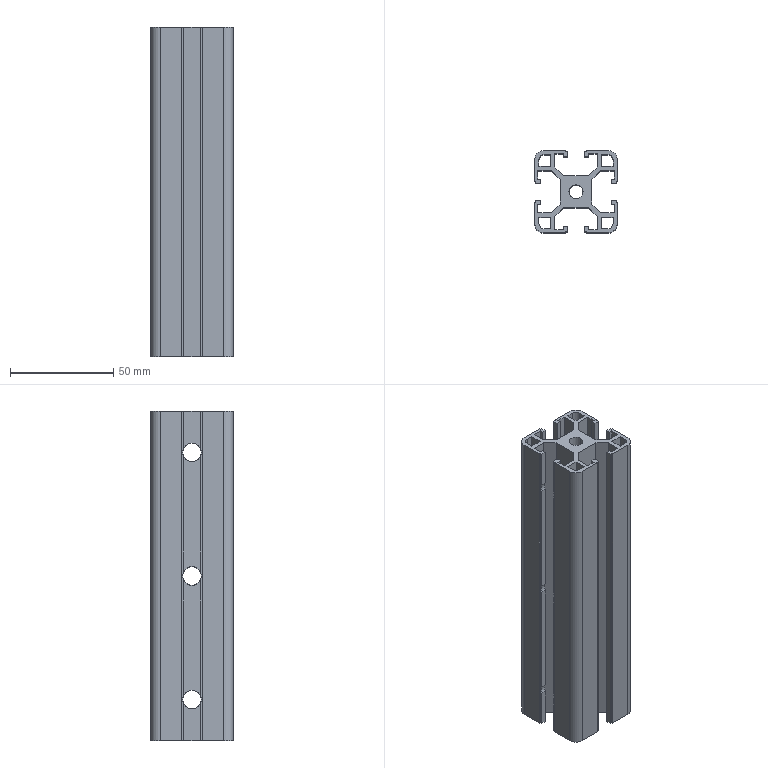Part | STEP file | 1 solid | 164 faces | box 40 x 40 x 160 mm | volume 89766 mm3 | plane 130 | cylinder 34 | commonest cylinder face diameters 9 x16 6.8 x8 15 x6 5 x4